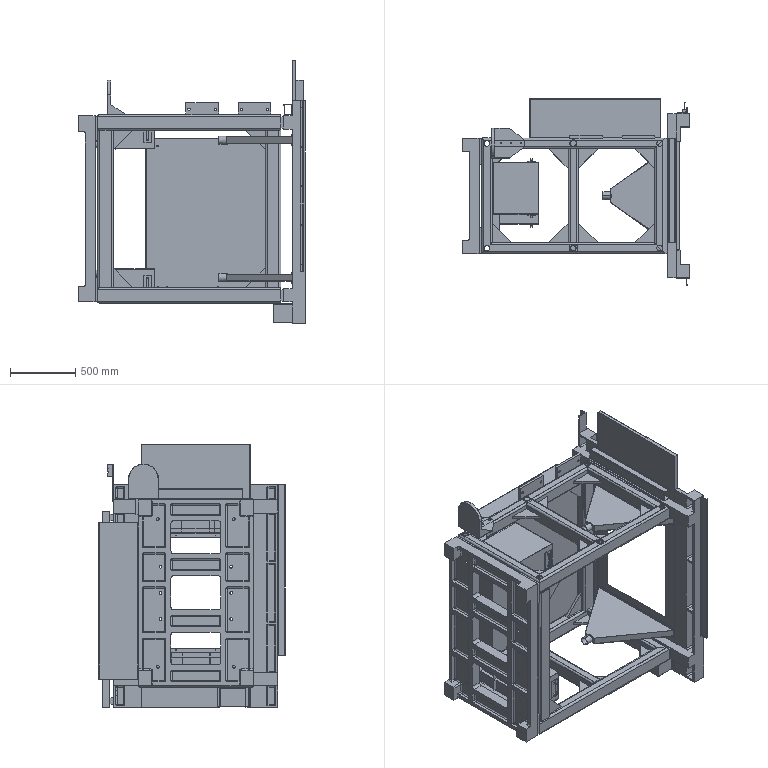Part | SolidWorks | features CompositeCurve 1 | 67 solids | 1920 faces | box 1731 x 1422 x 2008 mm | volume 170873319 mm3 | plane 969 | cylinder 743 | sphere 100 | cone 96 | torus 12 | commonest cylinder face diameters 20 x216 4.2 x96 5.5 x72 16 x52 32 x52 17.5 x40